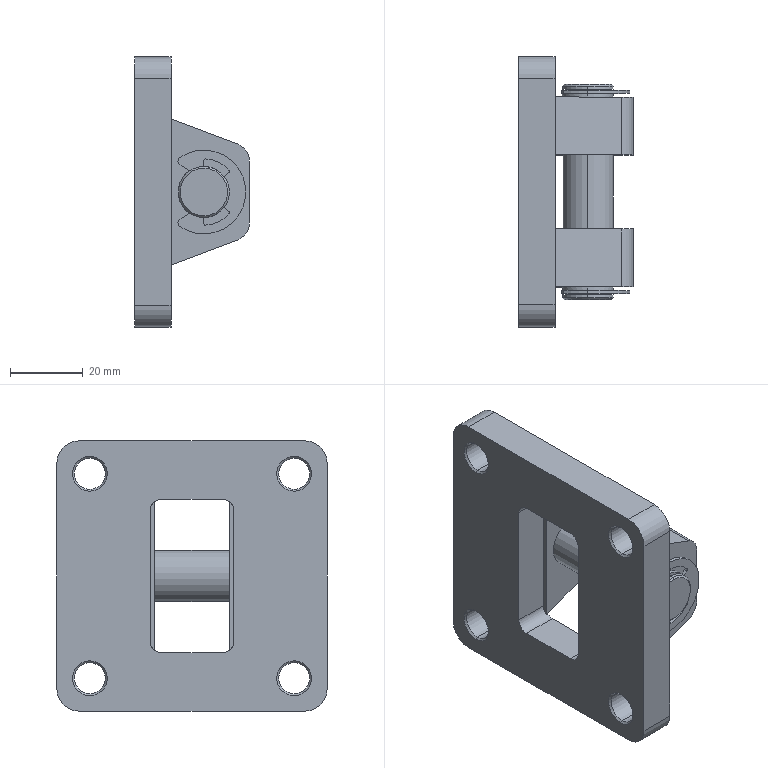Part | STEP file | F_SC63CB_F-SC63CB | 1 solid | 138 faces | box 31.5 x 74 x 74 mm | volume 67976 mm3 | cylinder 66 | plane 52 | cone 20 | commonest cylinder face diameters 1 x10 14 x10 8.5 x8 12 x8 13.5 x8 23 x6